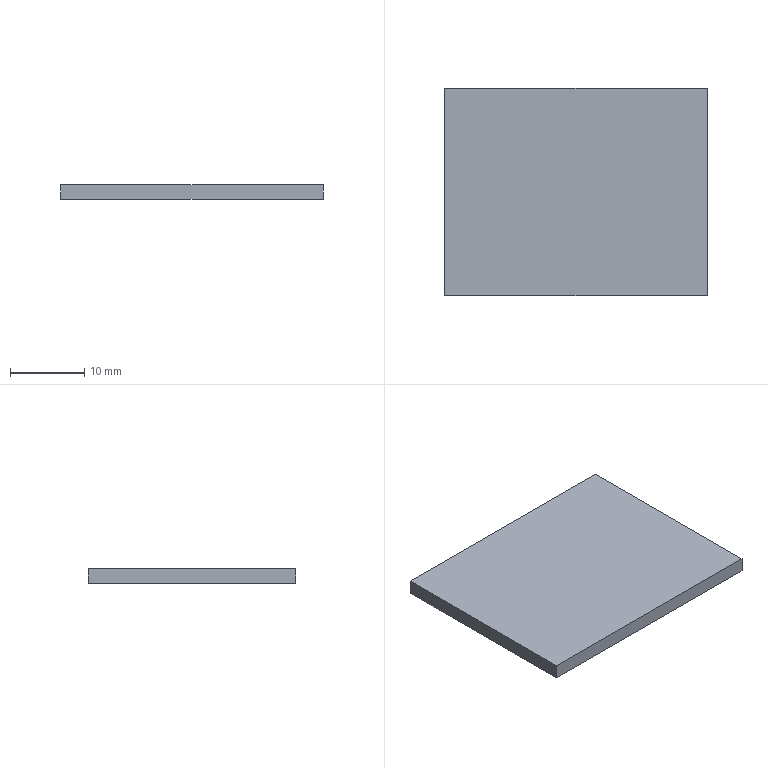Part | STEP file | SX-004-09 | 1 solid | 6 faces | box 35.36 x 28 x 2 mm | volume 1980 mm3 | plane 6
STEP:
#1=CARTESIAN_POINT('',(0.,0.,0.));
#2=DIRECTION('',(0.,0.,1.));
#3=DIRECTION('',(1.,0.,0.));
#4=AXIS2_PLACEMENT_3D('',#1,#2,#3);
#5=CARTESIAN_POINT('',(0.,28.,0.));
#6=VERTEX_POINT('',#5);
#7=CARTESIAN_POINT('',(0.,0.,0.));
#8=VERTEX_POINT('',#7);
#9=CARTESIAN_POINT('',(0.,0.,0.));
#10=DIRECTION('',(0.,-1.,0.));
#11=VECTOR('',#10,1.);
#12=LINE('',#9,#11);
#13=CARTESIAN_POINT('',(0.,0.,-2.));
#14=DIRECTION('',(-1.,0.,0.));
#15=DIRECTION('',(0.,-1.,0.));
#16=AXIS2_PLACEMENT_3D('',#13,#14,#15);
#17=PLANE('',#16);
#18=CARTESIAN_POINT('',(0.,2.));
#19=DIRECTION('',(1.,0.));
#20=VECTOR('',#19,1.);
#21=LINE('',#18,#20);
#22=(GEOMETRIC_REPRESENTATION_CONTEXT(2)PARAMETRIC_REPRESENTATION_CONTEXT()REPRESENTATION_CONTEXT('',''));
#23=DEFINITIONAL_REPRESENTATION('',(#21),#22);
#24=PCURVE('',#17,#23);
#25=CARTESIAN_POINT('',(0.,0.,0.));
#26=DIRECTION('',(0.,0.,-1.));
#27=DIRECTION('',(-1.,0.,0.));
#28=AXIS2_PLACEMENT_3D('',#25,#26,#27);
#29=PLANE('',#28);
#30=CARTESIAN_POINT('',(0.,0.));
#31=DIRECTION('',(0.,-1.));
#32=VECTOR('',#31,1.);
#33=LINE('',#30,#32);
#34=(GEOMETRIC_REPRESENTATION_CONTEXT(2)PARAMETRIC_REPRESENTATION_CONTEXT()REPRESENTATION_CONTEXT('',''));
#35=DEFINITIONAL_REPRESENTATION('',(#33),#34);
#36=PCURVE('',#29,#35);
#37=SURFACE_CURVE('',#12,(#24,#36),.PCURVE_S1.);
#38=EDGE_CURVE('',#6,#8,#37,.T.);
#39=ORIENTED_EDGE('',*,*,#38,.F.);
#40=CARTESIAN_POINT('',(0.,28.,-2.));
#41=VERTEX_POINT('',#40);
#42=CARTESIAN_POINT('',(0.,28.,-2.));
#43=DIRECTION('',(0.,0.,1.));
#44=VECTOR('',#43,1.);
#45=LINE('',#42,#44);
#46=CARTESIAN_POINT('',(-28.,0.));
#47=DIRECTION('',(0.,1.));
#48=VECTOR('',#47,1.);
#49=LINE('',#46,#48);
#50=(GEOMETRIC_REPRESENTATION_CONTEXT(2)PARAMETRIC_REPRESENTATION_CONTEXT()REPRESENTATION_CONTEXT('',''));
#51=DEFINITIONAL_REPRESENTATION('',(#49),#50);
#52=PCURVE('',#17,#51);
#53=CARTESIAN_POINT('',(0.,28.,-2.));
#54=DIRECTION('',(0.,1.,0.));
#55=DIRECTION('',(0.,0.,1.));
#56=AXIS2_PLACEMENT_3D('',#53,#54,#55);
#57=PLANE('',#56);
#58=CARTESIAN_POINT('',(0.,0.));
#59=DIRECTION('',(1.,0.));
#60=VECTOR('',#59,1.);
#61=LINE('',#58,#60);
#62=(GEOMETRIC_REPRESENTATION_CONTEXT(2)PARAMETRIC_REPRESENTATION_CONTEXT()REPRESENTATION_CONTEXT('',''));
#63=DEFINITIONAL_REPRESENTATION('',(#61),#62);
#64=PCURVE('',#57,#63);
#65=SURFACE_CURVE('',#45,(#52,#64),.PCURVE_S1.);
#66=EDGE_CURVE('',#41,#6,#65,.T.);
#67=ORIENTED_EDGE('',*,*,#66,.F.);
#68=CARTESIAN_POINT('',(0.,0.,-2.));
#69=VERTEX_POINT('',#68);
#70=CARTESIAN_POINT('',(0.,0.,-2.));
#71=DIRECTION('',(0.,-1.,0.));
#72=VECTOR('',#71,1.);
#73=LINE('',#70,#72);
#74=CARTESIAN_POINT('',(0.,0.));
#75=DIRECTION('',(1.,0.));
#76=VECTOR('',#75,1.);
#77=LINE('',#74,#76);
#78=(GEOMETRIC_REPRESENTATION_CONTEXT(2)PARAMETRIC_REPRESENTATION_CONTEXT()REPRESENTATION_CONTEXT('',''));
#79=DEFINITIONAL_REPRESENTATION('',(#77),#78);
#80=PCURVE('',#17,#79);
#81=CARTESIAN_POINT('',(0.,0.,-2.));
#82=DIRECTION('',(0.,0.,-1.));
#83=DIRECTION('',(-1.,0.,0.));
#84=AXIS2_PLACEMENT_3D('',#81,#82,#83);
#85=PLANE('',#84);
#86=CARTESIAN_POINT('',(0.,0.));
#87=DIRECTION('',(0.,-1.));
#88=VECTOR('',#87,1.);
#89=LINE('',#86,#88);
#90=(GEOMETRIC_REPRESENTATION_CONTEXT(2)PARAMETRIC_REPRESENTATION_CONTEXT()REPRESENTATION_CONTEXT('',''));
#91=DEFINITIONAL_REPRESENTATION('',(#89),#90);
#92=PCURVE('',#85,#91);
#93=SURFACE_CURVE('',#73,(#80,#92),.PCURVE_S1.);
#94=EDGE_CURVE('',#41,#69,#93,.T.);
#95=ORIENTED_EDGE('',*,*,#94,.T.);
#96=CARTESIAN_POINT('',(0.,0.,-2.));
#97=DIRECTION('',(0.,0.,1.));
#98=VECTOR('',#97,1.);
#99=LINE('',#96,#98);
#100=CARTESIAN_POINT('',(0.,0.));
#101=DIRECTION('',(0.,1.));
#102=VECTOR('',#101,1.);
#103=LINE('',#100,#102);
#104=(GEOMETRIC_REPRESENTATION_CONTEXT(2)PARAMETRIC_REPRESENTATION_CONTEXT()REPRESENTATION_CONTEXT('',''));
#105=DEFINITIONAL_REPRESENTATION('',(#103),#104);
#106=PCURVE('',#17,#105);
#107=CARTESIAN_POINT('',(0.,0.,-2.));
#108=DIRECTION('',(0.,-1.,0.));
#109=DIRECTION('',(0.,0.,-1.));
#110=AXIS2_PLACEMENT_3D('',#107,#108,#109);
#111=PLANE('',#110);
#112=CARTESIAN_POINT('',(0.,0.));
#113=DIRECTION('',(-1.,0.));
#114=VECTOR('',#113,1.);
#115=LINE('',#112,#114);
#116=(GEOMETRIC_REPRESENTATION_CONTEXT(2)PARAMETRIC_REPRESENTATION_CONTEXT()REPRESENTATION_CONTEXT('',''));
#117=DEFINITIONAL_REPRESENTATION('',(#115),#116);
#118=PCURVE('',#111,#117);
#119=SURFACE_CURVE('',#99,(#106,#118),.PCURVE_S1.);
#120=EDGE_CURVE('',#69,#8,#119,.T.);
#121=ORIENTED_EDGE('',*,*,#120,.T.);
#122=EDGE_LOOP('',(#39,#67,#95,#121));
#123=FACE_BOUND('',#122,.T.);
#124=ADVANCED_FACE('',(#123),#17,.T.);
#125=CARTESIAN_POINT('',(35.36,28.,0.));
#126=VERTEX_POINT('',#125);
#127=CARTESIAN_POINT('',(0.,28.,0.));
#128=DIRECTION('',(-1.,0.,0.));
#129=VECTOR('',#128,1.);
#130=LINE('',#127,#129);
#131=CARTESIAN_POINT('',(2.,0.));
#132=DIRECTION('',(0.,-1.));
#133=VECTOR('',#132,1.);
#134=LINE('',#131,#133);
#135=(GEOMETRIC_REPRESENTATION_CONTEXT(2)PARAMETRIC_REPRESENTATION_CONTEXT()REPRESENTATION_CONTEXT('',''));
#136=DEFINITIONAL_REPRESENTATION('',(#134),#135);
#137=PCURVE('',#57,#136);
#138=CARTESIAN_POINT('',(0.,28.));
#139=DIRECTION('',(1.,0.));
#140=VECTOR('',#139,1.);
#141=LINE('',#138,#140);
#142=(GEOMETRIC_REPRESENTATION_CONTEXT(2)PARAMETRIC_REPRESENTATION_CONTEXT()REPRESENTATION_CONTEXT('',''));
#143=DEFINITIONAL_REPRESENTATION('',(#141),#142);
#144=PCURVE('',#29,#143);
#145=SURFACE_CURVE('',#130,(#137,#144),.PCURVE_S1.);
#146=EDGE_CURVE('',#126,#6,#145,.T.);
#147=ORIENTED_EDGE('',*,*,#146,.F.);
#148=CARTESIAN_POINT('',(35.36,28.,-2.));
#149=VERTEX_POINT('',#148);
#150=CARTESIAN_POINT('',(35.36,28.,-2.));
#151=DIRECTION('',(0.,0.,1.));
#152=VECTOR('',#151,1.);
#153=LINE('',#150,#152);
#154=CARTESIAN_POINT('',(0.,35.36));
#155=DIRECTION('',(1.,0.));
#156=VECTOR('',#155,1.);
#157=LINE('',#154,#156);
#158=(GEOMETRIC_REPRESENTATION_CONTEXT(2)PARAMETRIC_REPRESENTATION_CONTEXT()REPRESENTATION_CONTEXT('',''));
#159=DEFINITIONAL_REPRESENTATION('',(#157),#158);
#160=PCURVE('',#57,#159);
#161=CARTESIAN_POINT('',(35.36,0.,-2.));
#162=DIRECTION('',(1.,0.,0.));
#163=DIRECTION('',(0.,1.,0.));
#164=AXIS2_PLACEMENT_3D('',#161,#162,#163);
#165=PLANE('',#164);
#166=CARTESIAN_POINT('',(28.,0.));
#167=DIRECTION('',(0.,1.));
#168=VECTOR('',#167,1.);
#169=LINE('',#166,#168);
#170=(GEOMETRIC_REPRESENTATION_CONTEXT(2)PARAMETRIC_REPRESENTATION_CONTEXT()REPRESENTATION_CONTEXT('',''));
#171=DEFINITIONAL_REPRESENTATION('',(#169),#170);
#172=PCURVE('',#165,#171);
#173=SURFACE_CURVE('',#153,(#160,#172),.PCURVE_S1.);
#174=EDGE_CURVE('',#149,#126,#173,.T.);
#175=ORIENTED_EDGE('',*,*,#174,.F.);
#176=CARTESIAN_POINT('',(0.,28.,-2.));
#177=DIRECTION('',(-1.,0.,0.));
#178=VECTOR('',#177,1.);
#179=LINE('',#176,#178);
#180=CARTESIAN_POINT('',(0.,0.));
#181=DIRECTION('',(0.,-1.));
#182=VECTOR('',#181,1.);
#183=LINE('',#180,#182);
#184=(GEOMETRIC_REPRESENTATION_CONTEXT(2)PARAMETRIC_REPRESENTATION_CONTEXT()REPRESENTATION_CONTEXT('',''));
#185=DEFINITIONAL_REPRESENTATION('',(#183),#184);
#186=PCURVE('',#57,#185);
#187=CARTESIAN_POINT('',(0.,28.));
#188=DIRECTION('',(1.,0.));
#189=VECTOR('',#188,1.);
#190=LINE('',#187,#189);
#191=(GEOMETRIC_REPRESENTATION_CONTEXT(2)PARAMETRIC_REPRESENTATION_CONTEXT()REPRESENTATION_CONTEXT('',''));
#192=DEFINITIONAL_REPRESENTATION('',(#190),#191);
#193=PCURVE('',#85,#192);
#194=SURFACE_CURVE('',#179,(#186,#193),.PCURVE_S1.);
#195=EDGE_CURVE('',#149,#41,#194,.T.);
#196=ORIENTED_EDGE('',*,*,#195,.T.);
#197=ORIENTED_EDGE('',*,*,#66,.T.);
#198=EDGE_LOOP('',(#147,#175,#196,#197));
#199=FACE_BOUND('',#198,.T.);
#200=ADVANCED_FACE('',(#199),#57,.T.);
#201=CARTESIAN_POINT('',(35.36,0.,0.));
#202=VERTEX_POINT('',#201);
#203=CARTESIAN_POINT('',(35.36,0.,0.));
#204=DIRECTION('',(0.,1.,0.));
#205=VECTOR('',#204,1.);
#206=LINE('',#203,#205);
#207=CARTESIAN_POINT('',(0.,2.));
#208=DIRECTION('',(1.,0.));
#209=VECTOR('',#208,1.);
#210=LINE('',#207,#209);
#211=(GEOMETRIC_REPRESENTATION_CONTEXT(2)PARAMETRIC_REPRESENTATION_CONTEXT()REPRESENTATION_CONTEXT('',''));
#212=DEFINITIONAL_REPRESENTATION('',(#210),#211);
#213=PCURVE('',#165,#212);
#214=CARTESIAN_POINT('',(-35.36,0.));
#215=DIRECTION('',(0.,1.));
#216=VECTOR('',#215,1.);
#217=LINE('',#214,#216);
#218=(GEOMETRIC_REPRESENTATION_CONTEXT(2)PARAMETRIC_REPRESENTATION_CONTEXT()REPRESENTATION_CONTEXT('',''));
#219=DEFINITIONAL_REPRESENTATION('',(#217),#218);
#220=PCURVE('',#29,#219);
#221=SURFACE_CURVE('',#206,(#213,#220),.PCURVE_S1.);
#222=EDGE_CURVE('',#202,#126,#221,.T.);
#223=ORIENTED_EDGE('',*,*,#222,.F.);
#224=CARTESIAN_POINT('',(35.36,0.,-2.));
#225=VERTEX_POINT('',#224);
#226=CARTESIAN_POINT('',(35.36,0.,-2.));
#227=DIRECTION('',(0.,0.,1.));
#228=VECTOR('',#227,1.);
#229=LINE('',#226,#228);
#230=CARTESIAN_POINT('',(0.,0.));
#231=DIRECTION('',(0.,1.));
#232=VECTOR('',#231,1.);
#233=LINE('',#230,#232);
#234=(GEOMETRIC_REPRESENTATION_CONTEXT(2)PARAMETRIC_REPRESENTATION_CONTEXT()REPRESENTATION_CONTEXT('',''));
#235=DEFINITIONAL_REPRESENTATION('',(#233),#234);
#236=PCURVE('',#165,#235);
#237=CARTESIAN_POINT('',(0.,35.36));
#238=DIRECTION('',(-1.,0.));
#239=VECTOR('',#238,1.);
#240=LINE('',#237,#239);
#241=(GEOMETRIC_REPRESENTATION_CONTEXT(2)PARAMETRIC_REPRESENTATION_CONTEXT()REPRESENTATION_CONTEXT('',''));
#242=DEFINITIONAL_REPRESENTATION('',(#240),#241);
#243=PCURVE('',#111,#242);
#244=SURFACE_CURVE('',#229,(#236,#243),.PCURVE_S1.);
#245=EDGE_CURVE('',#225,#202,#244,.T.);
#246=ORIENTED_EDGE('',*,*,#245,.F.);
#247=CARTESIAN_POINT('',(35.36,0.,-2.));
#248=DIRECTION('',(0.,1.,0.));
#249=VECTOR('',#248,1.);
#250=LINE('',#247,#249);
#251=CARTESIAN_POINT('',(0.,0.));
#252=DIRECTION('',(1.,0.));
#253=VECTOR('',#252,1.);
#254=LINE('',#251,#253);
#255=(GEOMETRIC_REPRESENTATION_CONTEXT(2)PARAMETRIC_REPRESENTATION_CONTEXT()REPRESENTATION_CONTEXT('',''));
#256=DEFINITIONAL_REPRESENTATION('',(#254),#255);
#257=PCURVE('',#165,#256);
#258=CARTESIAN_POINT('',(-35.36,0.));
#259=DIRECTION('',(0.,1.));
#260=VECTOR('',#259,1.);
#261=LINE('',#258,#260);
#262=(GEOMETRIC_REPRESENTATION_CONTEXT(2)PARAMETRIC_REPRESENTATION_CONTEXT()REPRESENTATION_CONTEXT('',''));
#263=DEFINITIONAL_REPRESENTATION('',(#261),#262);
#264=PCURVE('',#85,#263);
#265=SURFACE_CURVE('',#250,(#257,#264),.PCURVE_S1.);
#266=EDGE_CURVE('',#225,#149,#265,.T.);
#267=ORIENTED_EDGE('',*,*,#266,.T.);
#268=ORIENTED_EDGE('',*,*,#174,.T.);
#269=EDGE_LOOP('',(#223,#246,#267,#268));
#270=FACE_BOUND('',#269,.T.);
#271=ADVANCED_FACE('',(#270),#165,.T.);
#272=CARTESIAN_POINT('',(0.,0.,0.));
#273=DIRECTION('',(1.,0.,0.));
#274=VECTOR('',#273,1.);
#275=LINE('',#272,#274);
#276=CARTESIAN_POINT('',(-2.,0.));
#277=DIRECTION('',(0.,1.));
#278=VECTOR('',#277,1.);
#279=LINE('',#276,#278);
#280=(GEOMETRIC_REPRESENTATION_CONTEXT(2)PARAMETRIC_REPRESENTATION_CONTEXT()REPRESENTATION_CONTEXT('',''));
#281=DEFINITIONAL_REPRESENTATION('',(#279),#280);
#282=PCURVE('',#111,#281);
#283=CARTESIAN_POINT('',(0.,0.));
#284=DIRECTION('',(-1.,0.));
#285=VECTOR('',#284,1.);
#286=LINE('',#283,#285);
#287=(GEOMETRIC_REPRESENTATION_CONTEXT(2)PARAMETRIC_REPRESENTATION_CONTEXT()REPRESENTATION_CONTEXT('',''));
#288=DEFINITIONAL_REPRESENTATION('',(#286),#287);
#289=PCURVE('',#29,#288);
#290=SURFACE_CURVE('',#275,(#282,#289),.PCURVE_S1.);
#291=EDGE_CURVE('',#8,#202,#290,.T.);
#292=ORIENTED_EDGE('',*,*,#291,.F.);
#293=ORIENTED_EDGE('',*,*,#120,.F.);
#294=CARTESIAN_POINT('',(0.,0.,-2.));
#295=DIRECTION('',(1.,0.,0.));
#296=VECTOR('',#295,1.);
#297=LINE('',#294,#296);
#298=CARTESIAN_POINT('',(0.,0.));
#299=DIRECTION('',(0.,1.));
#300=VECTOR('',#299,1.);
#301=LINE('',#298,#300);
#302=(GEOMETRIC_REPRESENTATION_CONTEXT(2)PARAMETRIC_REPRESENTATION_CONTEXT()REPRESENTATION_CONTEXT('',''));
#303=DEFINITIONAL_REPRESENTATION('',(#301),#302);
#304=PCURVE('',#111,#303);
#305=CARTESIAN_POINT('',(0.,0.));
#306=DIRECTION('',(-1.,0.));
#307=VECTOR('',#306,1.);
#308=LINE('',#305,#307);
#309=(GEOMETRIC_REPRESENTATION_CONTEXT(2)PARAMETRIC_REPRESENTATION_CONTEXT()REPRESENTATION_CONTEXT('',''));
#310=DEFINITIONAL_REPRESENTATION('',(#308),#309);
#311=PCURVE('',#85,#310);
#312=SURFACE_CURVE('',#297,(#304,#311),.PCURVE_S1.);
#313=EDGE_CURVE('',#69,#225,#312,.T.);
#314=ORIENTED_EDGE('',*,*,#313,.T.);
#315=ORIENTED_EDGE('',*,*,#245,.T.);
#316=EDGE_LOOP('',(#292,#293,#314,#315));
#317=FACE_BOUND('',#316,.T.);
#318=ADVANCED_FACE('',(#317),#111,.T.);
#319=ORIENTED_EDGE('',*,*,#94,.F.);
#320=ORIENTED_EDGE('',*,*,#195,.F.);
#321=ORIENTED_EDGE('',*,*,#266,.F.);
#322=ORIENTED_EDGE('',*,*,#313,.F.);
#323=EDGE_LOOP('',(#319,#320,#321,#322));
#324=FACE_BOUND('',#323,.T.);
#325=ADVANCED_FACE('',(#324),#85,.T.);
#326=ORIENTED_EDGE('',*,*,#38,.T.);
#327=ORIENTED_EDGE('',*,*,#291,.T.);
#328=ORIENTED_EDGE('',*,*,#222,.T.);
#329=ORIENTED_EDGE('',*,*,#146,.T.);
#330=EDGE_LOOP('',(#326,#327,#328,#329));
#331=FACE_BOUND('',#330,.T.);
#332=ADVANCED_FACE('',(#331),#29,.F.);
#333=CLOSED_SHELL('',(#124,#200,#271,#318,#325,#332));
#334=MANIFOLD_SOLID_BREP('',#333);
#335=(LENGTH_UNIT()NAMED_UNIT(*)SI_UNIT(.MILLI.,.METRE.));
#336=UNCERTAINTY_MEASURE_WITH_UNIT(LENGTH_MEASURE(0.0000001),#335,'','');
#337=(NAMED_UNIT(*)PLANE_ANGLE_UNIT()SI_UNIT($,.RADIAN.));
#338=(NAMED_UNIT(*)SI_UNIT($,.STERADIAN.)SOLID_ANGLE_UNIT());
#339=(GEOMETRIC_REPRESENTATION_CONTEXT(3)GLOBAL_UNCERTAINTY_ASSIGNED_CONTEXT((#336))GLOBAL_UNIT_ASSIGNED_CONTEXT((#335,#337,#338))REPRESENTATION_CONTEXT('',''));
#340=ADVANCED_BREP_SHAPE_REPRESENTATION('',(#4,#334),#339);